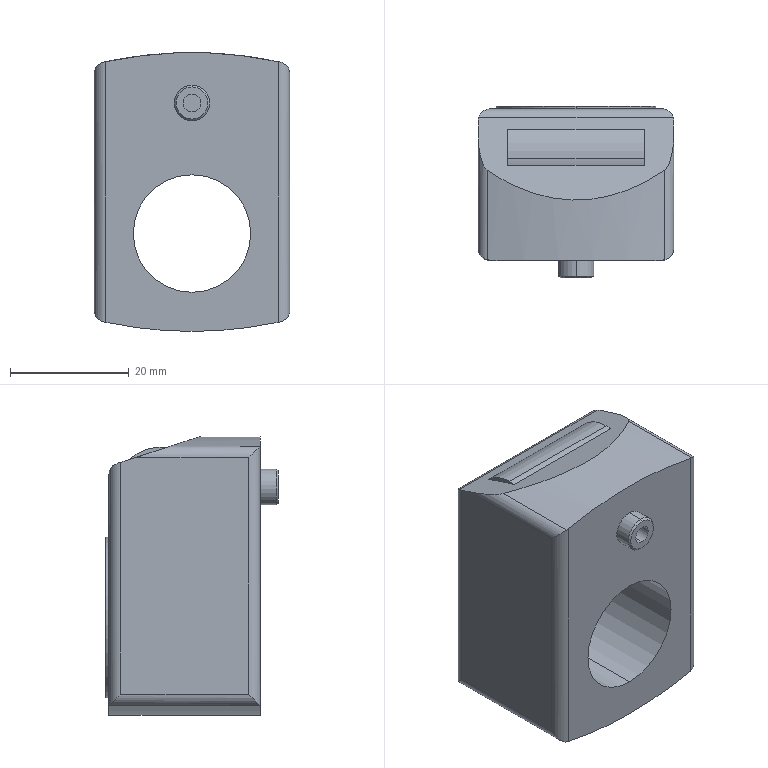Part | SolidWorks | features ICE 6, RefAxis 6, RevCut 3, 3DProfileFeature 2, Revolution 2, Extrusion 1 | 1 solid | 39 faces | box 33 x 29 x 47 mm | volume 29608 mm3 | cylinder 22 | plane 15 | cone 2 | commonest cylinder face diameters 4 x9 138.125 x3 3 x2 6 x2 14 x2 19.8 x2
STEP:
#1=CARTESIAN_POINT('',(11.5,3.069,28.669));
#2=VERTEX_POINT('',#1);
#3=CARTESIAN_POINT('',(11.5,2.,28.587));
#4=VERTEX_POINT('',#3);
#5=CARTESIAN_POINT('',(11.5,3.069,21.669));
#6=DIRECTION('',(1.,0.,0.));
#7=DIRECTION('',(0.,0.,-1.));
#8=AXIS2_PLACEMENT_3D('',#5,#6,#7);
#9=CIRCLE('',#8,7.);
#10=EDGE_CURVE('',#2,#4,#9,.T.);
#11=ORIENTED_EDGE('',*,*,#10,.F.);
#12=CARTESIAN_POINT('',(-11.5,3.069,28.669));
#13=VERTEX_POINT('',#12);
#14=CARTESIAN_POINT('',(11.5,3.069,28.669));
#15=DIRECTION('',(-1.,0.,0.));
#16=VECTOR('',#15,1000.);
#17=LINE('',#14,#16);
#18=EDGE_CURVE('',#2,#13,#17,.T.);
#19=ORIENTED_EDGE('',*,*,#18,.T.);
#20=CARTESIAN_POINT('',(-11.5,2.,28.587));
#21=VERTEX_POINT('',#20);
#22=CARTESIAN_POINT('',(-11.5,3.069,21.669));
#23=DIRECTION('',(1.,0.,0.));
#24=DIRECTION('',(0.,0.,-1.));
#25=AXIS2_PLACEMENT_3D('',#22,#23,#24);
#26=CIRCLE('',#25,7.);
#27=EDGE_CURVE('',#13,#21,#26,.T.);
#28=ORIENTED_EDGE('',*,*,#27,.T.);
#29=CARTESIAN_POINT('',(11.5,2.,28.587));
#30=DIRECTION('',(-1.,0.,0.));
#31=VECTOR('',#30,1000.);
#32=LINE('',#29,#31);
#33=EDGE_CURVE('',#4,#21,#32,.T.);
#34=ORIENTED_EDGE('',*,*,#33,.F.);
#35=EDGE_LOOP('',(#11,#19,#28,#34));
#36=FACE_OUTER_BOUND('',#35,.T.);
#37=CARTESIAN_POINT('',(11.5,3.069,21.669));
#38=DIRECTION('',(-1.,0.,0.));
#39=DIRECTION('',(0.,0.,1.));
#40=AXIS2_PLACEMENT_3D('',#37,#38,#39);
#41=CYLINDRICAL_SURFACE('',#40,7.);
#42=ADVANCED_FACE('',(#36),#41,.T.);
#43=CARTESIAN_POINT('',(0.,-17.,20.5));
#44=VERTEX_POINT('',#43);
#45=CARTESIAN_POINT('',(0.,-17.,23.5));
#46=VERTEX_POINT('',#45);
#47=CARTESIAN_POINT('',(0.,-17.,22.));
#48=DIRECTION('',(0.,1.,0.));
#49=DIRECTION('',(0.,0.,1.));
#50=AXIS2_PLACEMENT_3D('',#47,#48,#49);
#51=CIRCLE('',#50,1.5);
#52=EDGE_CURVE('',#44,#46,#51,.T.);
#53=ORIENTED_EDGE('',*,*,#52,.F.);
#54=CARTESIAN_POINT('',(0.,-12.,20.5));
#55=VERTEX_POINT('',#54);
#56=CARTESIAN_POINT('',(0.,-17.,20.5));
#57=DIRECTION('',(0.,1.,0.));
#58=VECTOR('',#57,1000.);
#59=LINE('',#56,#58);
#60=EDGE_CURVE('',#44,#55,#59,.T.);
#61=ORIENTED_EDGE('',*,*,#60,.T.);
#62=CARTESIAN_POINT('',(0.,-12.,23.5));
#63=VERTEX_POINT('',#62);
#64=CARTESIAN_POINT('',(0.,-12.,22.));
#65=DIRECTION('',(0.,1.,0.));
#66=DIRECTION('',(0.,0.,1.));
#67=AXIS2_PLACEMENT_3D('',#64,#65,#66);
#68=CIRCLE('',#67,1.5);
#69=EDGE_CURVE('',#55,#63,#68,.T.);
#70=ORIENTED_EDGE('',*,*,#69,.T.);
#71=CARTESIAN_POINT('',(0.,-17.,23.5));
#72=DIRECTION('',(0.,1.,0.));
#73=VECTOR('',#72,1000.);
#74=LINE('',#71,#73);
#75=EDGE_CURVE('',#46,#63,#74,.T.);
#76=ORIENTED_EDGE('',*,*,#75,.F.);
#77=EDGE_LOOP('',(#53,#61,#70,#76));
#78=FACE_OUTER_BOUND('',#77,.T.);
#79=CARTESIAN_POINT('',(0.,-17.,22.));
#80=DIRECTION('',(0.,1.,0.));
#81=DIRECTION('',(0.,0.,1.));
#82=AXIS2_PLACEMENT_3D('',#79,#80,#81);
#83=CYLINDRICAL_SURFACE('',#82,1.5);
#84=ADVANCED_FACE('',(#78),#83,.F.);
#85=CARTESIAN_POINT('',(0.,-17.,24.7));
#86=VERTEX_POINT('',#85);
#87=CARTESIAN_POINT('',(0.,-17.,19.3));
#88=VERTEX_POINT('',#87);
#89=CARTESIAN_POINT('',(0.,-17.,22.));
#90=DIRECTION('',(0.,1.,0.));
#91=DIRECTION('',(0.,0.,1.));
#92=AXIS2_PLACEMENT_3D('',#89,#90,#91);
#93=CIRCLE('',#92,2.7);
#94=EDGE_CURVE('',#86,#88,#93,.T.);
#95=ORIENTED_EDGE('',*,*,#94,.T.);
#96=CARTESIAN_POINT('',(0.,-16.7,19.));
#97=VERTEX_POINT('',#96);
#98=CARTESIAN_POINT('',(0.,-16.7,19.));
#99=DIRECTION('',(0.,0.7071,-0.7071));
#100=VECTOR('',#99,1000.);
#101=LINE('',#98,#100);
#102=EDGE_CURVE('',#88,#97,#101,.T.);
#103=ORIENTED_EDGE('',*,*,#102,.T.);
#104=CARTESIAN_POINT('',(0.,-16.7,25.));
#105=VERTEX_POINT('',#104);
#106=CARTESIAN_POINT('',(0.,-16.7,22.));
#107=DIRECTION('',(0.,1.,0.));
#108=DIRECTION('',(0.,0.,1.));
#109=AXIS2_PLACEMENT_3D('',#106,#107,#108);
#110=CIRCLE('',#109,3.);
#111=EDGE_CURVE('',#105,#97,#110,.T.);
#112=ORIENTED_EDGE('',*,*,#111,.F.);
#113=CARTESIAN_POINT('',(0.,-16.7,25.));
#114=DIRECTION('',(0.,0.7071,0.7071));
#115=VECTOR('',#114,1000.);
#116=LINE('',#113,#115);
#117=EDGE_CURVE('',#86,#105,#116,.T.);
#118=ORIENTED_EDGE('',*,*,#117,.F.);
#119=EDGE_LOOP('',(#95,#103,#112,#118));
#120=FACE_OUTER_BOUND('',#119,.T.);
#121=CARTESIAN_POINT('',(0.,-16.7,22.));
#122=DIRECTION('',(0.,1.,0.));
#123=DIRECTION('',(0.,0.,1.));
#124=AXIS2_PLACEMENT_3D('',#121,#122,#123);
#125=CONICAL_SURFACE('',#124,3.,0.7854);
#126=ADVANCED_FACE('',(#120),#125,.T.);
#127=ORIENTED_EDGE('',*,*,#111,.T.);
#128=CARTESIAN_POINT('',(0.,-14.,19.));
#129=VERTEX_POINT('',#128);
#130=CARTESIAN_POINT('',(0.,-10.,19.));
#131=DIRECTION('',(0.,1.,0.));
#132=VECTOR('',#131,1000.);
#133=LINE('',#130,#132);
#134=EDGE_CURVE('',#97,#129,#133,.T.);
#135=ORIENTED_EDGE('',*,*,#134,.T.);
#136=CARTESIAN_POINT('',(0.,-14.,25.));
#137=VERTEX_POINT('',#136);
#138=CARTESIAN_POINT('',(0.,-14.,22.));
#139=DIRECTION('',(0.,1.,0.));
#140=DIRECTION('',(0.,0.,1.));
#141=AXIS2_PLACEMENT_3D('',#138,#139,#140);
#142=CIRCLE('',#141,3.);
#143=EDGE_CURVE('',#137,#129,#142,.T.);
#144=ORIENTED_EDGE('',*,*,#143,.F.);
#145=CARTESIAN_POINT('',(0.,-10.,25.));
#146=DIRECTION('',(0.,1.,0.));
#147=VECTOR('',#146,1000.);
#148=LINE('',#145,#147);
#149=EDGE_CURVE('',#105,#137,#148,.T.);
#150=ORIENTED_EDGE('',*,*,#149,.F.);
#151=EDGE_LOOP('',(#127,#135,#144,#150));
#152=FACE_OUTER_BOUND('',#151,.T.);
#153=CARTESIAN_POINT('',(0.,-10.,22.));
#154=DIRECTION('',(0.,1.,0.));
#155=DIRECTION('',(0.,0.,1.));
#156=AXIS2_PLACEMENT_3D('',#153,#154,#155);
#157=CYLINDRICAL_SURFACE('',#156,3.);
#158=ADVANCED_FACE('',(#152),#157,.T.);
#159=CARTESIAN_POINT('',(0.,11.5,13.5));
#160=VERTEX_POINT('',#159);
#161=CARTESIAN_POINT('',(0.,11.5,-13.5));
#162=VERTEX_POINT('',#161);
#163=CARTESIAN_POINT('',(0.,11.5,0.));
#164=DIRECTION('',(0.,1.,0.));
#165=DIRECTION('',(0.,0.,1.));
#166=AXIS2_PLACEMENT_3D('',#163,#164,#165);
#167=CIRCLE('',#166,13.5);
#168=EDGE_CURVE('',#160,#162,#167,.T.);
#169=ORIENTED_EDGE('',*,*,#168,.T.);
#170=CARTESIAN_POINT('',(0.,12.,-13.5));
#171=VERTEX_POINT('',#170);
#172=CARTESIAN_POINT('',(0.,5.,-13.5));
#173=DIRECTION('',(0.,1.,0.));
#174=VECTOR('',#173,1000.);
#175=LINE('',#172,#174);
#176=EDGE_CURVE('',#162,#171,#175,.T.);
#177=ORIENTED_EDGE('',*,*,#176,.T.);
#178=CARTESIAN_POINT('',(0.,12.,13.5));
#179=VERTEX_POINT('',#178);
#180=CARTESIAN_POINT('',(0.,12.,0.));
#181=DIRECTION('',(0.,1.,0.));
#182=DIRECTION('',(0.,0.,1.));
#183=AXIS2_PLACEMENT_3D('',#180,#181,#182);
#184=CIRCLE('',#183,13.5);
#185=EDGE_CURVE('',#179,#171,#184,.T.);
#186=ORIENTED_EDGE('',*,*,#185,.F.);
#187=CARTESIAN_POINT('',(0.,5.,13.5));
#188=DIRECTION('',(0.,1.,0.));
#189=VECTOR('',#188,1000.);
#190=LINE('',#187,#189);
#191=EDGE_CURVE('',#160,#179,#190,.T.);
#192=ORIENTED_EDGE('',*,*,#191,.F.);
#193=EDGE_LOOP('',(#169,#177,#186,#192));
#194=FACE_OUTER_BOUND('',#193,.T.);
#195=CARTESIAN_POINT('',(0.,5.,0.));
#196=DIRECTION('',(0.,1.,0.));
#197=DIRECTION('',(0.,0.,1.));
#198=AXIS2_PLACEMENT_3D('',#195,#196,#197);
#199=CYLINDRICAL_SURFACE('',#198,13.5);
#200=ADVANCED_FACE('',(#194),#199,.T.);
#201=CARTESIAN_POINT('',(0.,-14.,9.9));
#202=VERTEX_POINT('',#201);
#203=CARTESIAN_POINT('',(0.,-14.,-9.9));
#204=VERTEX_POINT('',#203);
#205=CARTESIAN_POINT('',(0.,-14.,0.));
#206=DIRECTION('',(0.,-1.,0.));
#207=DIRECTION('',(0.,0.,-1.));
#208=AXIS2_PLACEMENT_3D('',#205,#206,#207);
#209=CIRCLE('',#208,9.9);
#210=EDGE_CURVE('',#202,#204,#209,.T.);
#211=ORIENTED_EDGE('',*,*,#210,.T.);
#212=CARTESIAN_POINT('',(0.,12.,-9.9));
#213=VERTEX_POINT('',#212);
#214=CARTESIAN_POINT('',(0.,12.,-9.9));
#215=DIRECTION('',(0.,1.,0.));
#216=VECTOR('',#215,1000.);
#217=LINE('',#214,#216);
#218=EDGE_CURVE('',#204,#213,#217,.T.);
#219=ORIENTED_EDGE('',*,*,#218,.T.);
#220=CARTESIAN_POINT('',(0.,12.,9.9));
#221=VERTEX_POINT('',#220);
#222=CARTESIAN_POINT('',(0.,12.,0.));
#223=DIRECTION('',(0.,1.,0.));
#224=DIRECTION('',(0.,0.,1.));
#225=AXIS2_PLACEMENT_3D('',#222,#223,#224);
#226=CIRCLE('',#225,9.9);
#227=EDGE_CURVE('',#213,#221,#226,.T.);
#228=ORIENTED_EDGE('',*,*,#227,.T.);
#229=CARTESIAN_POINT('',(0.,12.,9.9));
#230=DIRECTION('',(0.,1.,0.));
#231=VECTOR('',#230,1000.);
#232=LINE('',#229,#231);
#233=EDGE_CURVE('',#202,#221,#232,.T.);
#234=ORIENTED_EDGE('',*,*,#233,.F.);
#235=EDGE_LOOP('',(#211,#219,#228,#234));
#236=FACE_OUTER_BOUND('',#235,.T.);
#237=CARTESIAN_POINT('',(0.,12.,0.));
#238=DIRECTION('',(0.,1.,0.));
#239=DIRECTION('',(0.,0.,1.));
#240=AXIS2_PLACEMENT_3D('',#237,#238,#239);
#241=CYLINDRICAL_SURFACE('',#240,9.9);
#242=ADVANCED_FACE('',(#236),#241,.F.);
#243=CARTESIAN_POINT('',(0.,11.5,-16.5));
#244=VERTEX_POINT('',#243);
#245=CARTESIAN_POINT('',(-14.5,11.5,-14.961));
#246=VERTEX_POINT('',#245);
#247=CARTESIAN_POINT('',(0.,11.5,52.563));
#248=DIRECTION('',(0.,1.,0.));
#249=DIRECTION('',(0.,0.,1.));
#250=AXIS2_PLACEMENT_3D('',#247,#248,#249);
#251=CIRCLE('',#250,69.063);
#252=EDGE_CURVE('',#244,#246,#251,.T.);
#253=ORIENTED_EDGE('',*,*,#252,.F.);
#254=CARTESIAN_POINT('',(0.,-14.,-16.5));
#255=VERTEX_POINT('',#254);
#256=CARTESIAN_POINT('',(0.,11.5,-16.5));
#257=DIRECTION('',(0.,-1.,0.));
#258=VECTOR('',#257,1000.);
#259=LINE('',#256,#258);
#260=EDGE_CURVE('',#244,#255,#259,.T.);
#261=ORIENTED_EDGE('',*,*,#260,.T.);
#262=CARTESIAN_POINT('',(-14.5,-14.,-14.961));
#263=VERTEX_POINT('',#262);
#264=CARTESIAN_POINT('',(0.,-14.,52.563));
#265=DIRECTION('',(0.,1.,0.));
#266=DIRECTION('',(0.,0.,1.));
#267=AXIS2_PLACEMENT_3D('',#264,#265,#266);
#268=CIRCLE('',#267,69.063);
#269=EDGE_CURVE('',#255,#263,#268,.T.);
#270=ORIENTED_EDGE('',*,*,#269,.T.);
#271=CARTESIAN_POINT('',(-14.932,-13.953,-14.866));
#272=VERTEX_POINT('',#271);
#273=CARTESIAN_POINT('',(-14.932,-13.953,-14.866));
#274=CARTESIAN_POINT('',(-14.79,-13.984,-14.898));
#275=CARTESIAN_POINT('',(-14.646,-14.,-14.929));
#276=CARTESIAN_POINT('',(-14.5,-14.,-14.961));
#277=B_SPLINE_CURVE_WITH_KNOTS('',3,(#273,#274,#275,#276),.UNSPECIFIED.,.F.,.F.,(4,4),(0.,0.0004451),.UNSPECIFIED.);
#278=EDGE_CURVE('',#272,#263,#277,.T.);
#279=ORIENTED_EDGE('',*,*,#278,.F.);
#280=CARTESIAN_POINT('',(-14.932,11.453,-14.866));
#281=VERTEX_POINT('',#280);
#282=CARTESIAN_POINT('',(-14.932,11.5,-14.866));
#283=DIRECTION('',(0.,-1.,0.));
#284=VECTOR('',#283,1000.);
#285=LINE('',#282,#284);
#286=EDGE_CURVE('',#281,#272,#285,.T.);
#287=ORIENTED_EDGE('',*,*,#286,.F.);
#288=CARTESIAN_POINT('',(-14.5,11.5,-14.961));
#289=CARTESIAN_POINT('',(-14.646,11.5,-14.929));
#290=CARTESIAN_POINT('',(-14.79,11.484,-14.898));
#291=CARTESIAN_POINT('',(-14.932,11.453,-14.866));
#292=B_SPLINE_CURVE_WITH_KNOTS('',3,(#288,#289,#290,#291),.UNSPECIFIED.,.F.,.F.,(4,4),(0.,0.0004451),.UNSPECIFIED.);
#293=EDGE_CURVE('',#246,#281,#292,.T.);
#294=ORIENTED_EDGE('',*,*,#293,.F.);
#295=EDGE_LOOP('',(#253,#261,#270,#279,#287,#294));
#296=FACE_OUTER_BOUND('',#295,.T.);
#297=CARTESIAN_POINT('',(0.,11.5,52.563));
#298=DIRECTION('',(0.,-1.,0.));
#299=DIRECTION('',(0.,0.,-1.));
#300=AXIS2_PLACEMENT_3D('',#297,#298,#299);
#301=CYLINDRICAL_SURFACE('',#300,69.063);
#302=ADVANCED_FACE('',(#296),#301,.T.);
#303=ORIENTED_EDGE('',*,*,#94,.F.);
#304=CARTESIAN_POINT('',(0.,-17.,22.));
#305=DIRECTION('',(0.,1.,0.));
#306=DIRECTION('',(0.,0.,1.));
#307=AXIS2_PLACEMENT_3D('',#304,#305,#306);
#308=CIRCLE('',#307,2.7);
#309=EDGE_CURVE('',#88,#86,#308,.T.);
#310=ORIENTED_EDGE('',*,*,#309,.F.);
#311=EDGE_LOOP('',(#303,#310));
#312=FACE_OUTER_BOUND('',#311,.T.);
#313=CARTESIAN_POINT('',(0.,-17.,22.));
#314=DIRECTION('',(0.,1.,0.));
#315=DIRECTION('',(0.,0.,1.));
#316=AXIS2_PLACEMENT_3D('',#313,#314,#315);
#317=CIRCLE('',#316,1.5);
#318=EDGE_CURVE('',#46,#44,#317,.T.);
#319=ORIENTED_EDGE('',*,*,#318,.T.);
#320=ORIENTED_EDGE('',*,*,#52,.T.);
#321=EDGE_LOOP('',(#319,#320));
#322=FACE_BOUND('',#321,.T.);
#323=CARTESIAN_POINT('',(0.,-17.,22.));
#324=DIRECTION('',(0.,-1.,0.));
#325=DIRECTION('',(0.,0.,-1.));
#326=AXIS2_PLACEMENT_3D('',#323,#324,#325);
#327=PLANE('',#326);
#328=ADVANCED_FACE('',(#312,#322),#327,.T.);
#329=ORIENTED_EDGE('',*,*,#143,.T.);
#330=CARTESIAN_POINT('',(0.,-14.,22.));
#331=DIRECTION('',(0.,1.,0.));
#332=DIRECTION('',(0.,0.,1.));
#333=AXIS2_PLACEMENT_3D('',#330,#331,#332);
#334=CIRCLE('',#333,3.);
#335=EDGE_CURVE('',#129,#137,#334,.T.);
#336=ORIENTED_EDGE('',*,*,#335,.T.);
#337=EDGE_LOOP('',(#329,#336));
#338=FACE_BOUND('',#337,.T.);
#339=CARTESIAN_POINT('',(14.5,-14.,-14.961));
#340=VERTEX_POINT('',#339);
#341=CARTESIAN_POINT('',(14.5,-14.,28.961));
#342=VERTEX_POINT('',#341);
#343=CARTESIAN_POINT('',(14.5,-14.,-35.));
#344=DIRECTION('',(0.,0.,1.));
#345=VECTOR('',#344,1000.);
#346=LINE('',#343,#345);
#347=EDGE_CURVE('',#340,#342,#346,.T.);
#348=ORIENTED_EDGE('',*,*,#347,.T.);
#349=CARTESIAN_POINT('',(-14.5,-14.,28.961));
#350=VERTEX_POINT('',#349);
#351=CARTESIAN_POINT('',(0.,-14.,-38.563));
#352=DIRECTION('',(0.,1.,0.));
#353=DIRECTION('',(0.,0.,1.));
#354=AXIS2_PLACEMENT_3D('',#351,#352,#353);
#355=CIRCLE('',#354,69.063);
#356=EDGE_CURVE('',#350,#342,#355,.T.);
#357=ORIENTED_EDGE('',*,*,#356,.F.);
#358=CARTESIAN_POINT('',(-14.5,-14.,-35.));
#359=DIRECTION('',(0.,0.,1.));
#360=VECTOR('',#359,1000.);
#361=LINE('',#358,#360);
#362=EDGE_CURVE('',#263,#350,#361,.T.);
#363=ORIENTED_EDGE('',*,*,#362,.F.);
#364=ORIENTED_EDGE('',*,*,#269,.F.);
#365=CARTESIAN_POINT('',(0.,-14.,52.563));
#366=DIRECTION('',(0.,1.,0.));
#367=DIRECTION('',(0.,0.,1.));
#368=AXIS2_PLACEMENT_3D('',#365,#366,#367);
#369=CIRCLE('',#368,69.063);
#370=EDGE_CURVE('',#340,#255,#369,.T.);
#371=ORIENTED_EDGE('',*,*,#370,.F.);
#372=EDGE_LOOP('',(#348,#357,#363,#364,#371));
#373=FACE_OUTER_BOUND('',#372,.T.);
#374=ORIENTED_EDGE('',*,*,#210,.F.);
#375=CARTESIAN_POINT('',(0.,-14.,0.));
#376=DIRECTION('',(0.,-1.,0.));
#377=DIRECTION('',(0.,0.,-1.));
#378=AXIS2_PLACEMENT_3D('',#375,#376,#377);
#379=CIRCLE('',#378,9.9);
#380=EDGE_CURVE('',#204,#202,#379,.T.);
#381=ORIENTED_EDGE('',*,*,#380,.F.);
#382=EDGE_LOOP('',(#374,#381));
#383=FACE_BOUND('',#382,.T.);
#384=CARTESIAN_POINT('',(-14.5,-14.,-12.914));
#385=DIRECTION('',(0.,1.,0.));
#386=DIRECTION('',(0.,0.,1.));
#387=AXIS2_PLACEMENT_3D('',#384,#385,#386);
#388=PLANE('',#387);
#389=ADVANCED_FACE('',(#338,#373,#383),#388,.F.);
#390=CARTESIAN_POINT('',(-16.5,9.5,-12.914));
#391=VERTEX_POINT('',#390);
#392=CARTESIAN_POINT('',(-14.932,11.453,-14.866));
#393=CARTESIAN_POINT('',(-15.888,11.241,-14.655));
#394=CARTESIAN_POINT('',(-16.5,10.478,-13.892));
#395=CARTESIAN_POINT('',(-16.5,9.5,-12.914));
#396=(BOUNDED_CURVE()B_SPLINE_CURVE(3,(#392,#393,#394,#395),.UNSPECIFIED.,.F.,.F.)B_SPLINE_CURVE_WITH_KNOTS((4,4),(3.36,4.712),.UNSPECIFIED.)CURVE()GEOMETRIC_REPRESENTATION_ITEM()RATIONAL_B_SPLINE_CURVE((1.,0.8532,0.8532,1.))REPRESENTATION_ITEM(''));
#397=EDGE_CURVE('',#281,#391,#396,.T.);
#398=ORIENTED_EDGE('',*,*,#397,.F.);
#399=ORIENTED_EDGE('',*,*,#286,.T.);
#400=CARTESIAN_POINT('',(-16.5,-12.,-12.914));
#401=VERTEX_POINT('',#400);
#402=CARTESIAN_POINT('',(-16.5,-12.,-12.914));
#403=CARTESIAN_POINT('',(-16.5,-12.978,-13.892));
#404=CARTESIAN_POINT('',(-15.888,-13.741,-14.655));
#405=CARTESIAN_POINT('',(-14.932,-13.953,-14.866));
#406=(BOUNDED_CURVE()B_SPLINE_CURVE(3,(#402,#403,#404,#405),.UNSPECIFIED.,.F.,.F.)B_SPLINE_CURVE_WITH_KNOTS((4,4),(4.712,6.065),.UNSPECIFIED.)CURVE()GEOMETRIC_REPRESENTATION_ITEM()RATIONAL_B_SPLINE_CURVE((1.,0.8532,0.8532,1.))REPRESENTATION_ITEM(''));
#407=EDGE_CURVE('',#401,#272,#406,.T.);
#408=ORIENTED_EDGE('',*,*,#407,.F.);
#409=CARTESIAN_POINT('',(-16.5,11.5,-12.914));
#410=DIRECTION('',(0.,-1.,0.));
#411=VECTOR('',#410,1000.);
#412=LINE('',#409,#411);
#413=EDGE_CURVE('',#391,#401,#412,.T.);
#414=ORIENTED_EDGE('',*,*,#413,.F.);
#415=EDGE_LOOP('',(#398,#399,#408,#414));
#416=FACE_OUTER_BOUND('',#415,.T.);
#417=CARTESIAN_POINT('',(-14.5,11.5,-12.914));
#418=DIRECTION('',(0.,-1.,0.));
#419=DIRECTION('',(0.,0.,-1.));
#420=AXIS2_PLACEMENT_3D('',#417,#418,#419);
#421=CYLINDRICAL_SURFACE('',#420,2.);
#422=ADVANCED_FACE('',(#416),#421,.T.);
#423=CARTESIAN_POINT('',(-16.5,7.149,26.914));
#424=VERTEX_POINT('',#423);
#425=CARTESIAN_POINT('',(-16.5,-12.,26.914));
#426=VERTEX_POINT('',#425);
#427=CARTESIAN_POINT('',(-16.5,11.5,26.914));
#428=DIRECTION('',(0.,-1.,0.));
#429=VECTOR('',#428,1000.);
#430=LINE('',#427,#429);
#431=EDGE_CURVE('',#424,#426,#430,.T.);
#432=ORIENTED_EDGE('',*,*,#431,.F.);
#433=CARTESIAN_POINT('',(-16.5,9.5,26.15));
#434=VERTEX_POINT('',#433);
#435=CARTESIAN_POINT('',(-16.5,22.789,21.832));
#436=DIRECTION('',(0.,0.9511,-0.309));
#437=VECTOR('',#436,1000.);
#438=LINE('',#435,#437);
#439=EDGE_CURVE('',#424,#434,#438,.T.);
#440=ORIENTED_EDGE('',*,*,#439,.T.);
#441=CARTESIAN_POINT('',(-16.5,9.5,-35.));
#442=DIRECTION('',(0.,0.,1.));
#443=VECTOR('',#442,1000.);
#444=LINE('',#441,#443);
#445=EDGE_CURVE('',#391,#434,#444,.T.);
#446=ORIENTED_EDGE('',*,*,#445,.F.);
#447=ORIENTED_EDGE('',*,*,#413,.T.);
#448=CARTESIAN_POINT('',(-16.5,-12.,-35.));
#449=DIRECTION('',(0.,0.,1.));
#450=VECTOR('',#449,1000.);
#451=LINE('',#448,#450);
#452=EDGE_CURVE('',#401,#426,#451,.T.);
#453=ORIENTED_EDGE('',*,*,#452,.T.);
#454=EDGE_LOOP('',(#432,#440,#446,#447,#453));
#455=FACE_OUTER_BOUND('',#454,.T.);
#456=CARTESIAN_POINT('',(-16.5,11.5,-12.914));
#457=DIRECTION('',(1.,0.,0.));
#458=DIRECTION('',(0.,0.,-1.));
#459=AXIS2_PLACEMENT_3D('',#456,#457,#458);
#460=PLANE('',#459);
#461=ADVANCED_FACE('',(#455),#460,.F.);
#462=CARTESIAN_POINT('',(-14.932,1.139,28.866));
#463=VERTEX_POINT('',#462);
#464=CARTESIAN_POINT('',(-14.932,-13.953,28.866));
#465=VERTEX_POINT('',#464);
#466=CARTESIAN_POINT('',(-14.932,11.5,28.866));
#467=DIRECTION('',(0.,-1.,0.));
#468=VECTOR('',#467,1000.);
#469=LINE('',#466,#468);
#470=EDGE_CURVE('',#463,#465,#469,.T.);
#471=ORIENTED_EDGE('',*,*,#470,.F.);
#472=CARTESIAN_POINT('',(-14.932,1.139,28.866));
#473=CARTESIAN_POINT('',(-15.888,1.79,28.655));
#474=CARTESIAN_POINT('',(-16.5,4.138,27.892));
#475=CARTESIAN_POINT('',(-16.5,7.149,26.914));
#476=(BOUNDED_CURVE()B_SPLINE_CURVE(3,(#472,#473,#474,#475),.UNSPECIFIED.,.F.,.F.)B_SPLINE_CURVE_WITH_KNOTS((4,4),(0.2179,1.571),.UNSPECIFIED.)CURVE()GEOMETRIC_REPRESENTATION_ITEM()RATIONAL_B_SPLINE_CURVE((1.,0.8532,0.8532,1.))REPRESENTATION_ITEM(''));
#477=EDGE_CURVE('',#463,#424,#476,.T.);
#478=ORIENTED_EDGE('',*,*,#477,.T.);
#479=ORIENTED_EDGE('',*,*,#431,.T.);
#480=CARTESIAN_POINT('',(-14.932,-13.953,28.866));
#481=CARTESIAN_POINT('',(-15.888,-13.741,28.655));
#482=CARTESIAN_POINT('',(-16.5,-12.978,27.892));
#483=CARTESIAN_POINT('',(-16.5,-12.,26.914));
#484=(BOUNDED_CURVE()B_SPLINE_CURVE(3,(#480,#481,#482,#483),.UNSPECIFIED.,.F.,.F.)B_SPLINE_CURVE_WITH_KNOTS((4,4),(0.2179,1.571),.UNSPECIFIED.)CURVE()GEOMETRIC_REPRESENTATION_ITEM()RATIONAL_B_SPLINE_CURVE((1.,0.8532,0.8532,1.))REPRESENTATION_ITEM(''));
#485=EDGE_CURVE('',#465,#426,#484,.T.);
#486=ORIENTED_EDGE('',*,*,#485,.F.);
#487=EDGE_LOOP('',(#471,#478,#479,#486));
#488=FACE_OUTER_BOUND('',#487,.T.);
#489=CARTESIAN_POINT('',(-14.5,11.5,26.914));
#490=DIRECTION('',(0.,-1.,0.));
#491=DIRECTION('',(0.,0.,-1.));
#492=AXIS2_PLACEMENT_3D('',#489,#490,#491);
#493=CYLINDRICAL_SURFACE('',#492,2.);
#494=ADVANCED_FACE('',(#488),#493,.T.);
#495=CARTESIAN_POINT('',(14.932,1.139,28.866));
#496=VERTEX_POINT('',#495);
#497=CARTESIAN_POINT('',(14.932,-13.953,28.866));
#498=VERTEX_POINT('',#497);
#499=CARTESIAN_POINT('',(14.932,11.5,28.866));
#500=DIRECTION('',(0.,-1.,0.));
#501=VECTOR('',#500,1000.);
#502=LINE('',#499,#501);
#503=EDGE_CURVE('',#496,#498,#502,.T.);
#504=ORIENTED_EDGE('',*,*,#503,.F.);
#505=CARTESIAN_POINT('',(14.932,1.139,28.866));
#506=CARTESIAN_POINT('',(5.057,-5.591,31.053));
#507=CARTESIAN_POINT('',(-5.057,-5.591,31.053));
#508=CARTESIAN_POINT('',(-14.932,1.139,28.866));
#509=(BOUNDED_CURVE()B_SPLINE_CURVE(3,(#505,#506,#507,#508),.UNSPECIFIED.,.F.,.F.)B_SPLINE_CURVE_WITH_KNOTS((4,4),(6.065,6.501),.UNSPECIFIED.)CURVE()GEOMETRIC_REPRESENTATION_ITEM()RATIONAL_B_SPLINE_CURVE((1.,0.9842,0.9842,1.))REPRESENTATION_ITEM(''));
#510=EDGE_CURVE('',#496,#463,#509,.T.);
#511=ORIENTED_EDGE('',*,*,#510,.T.);
#512=ORIENTED_EDGE('',*,*,#470,.T.);
#513=CARTESIAN_POINT('',(-14.5,-14.,28.961));
#514=CARTESIAN_POINT('',(-14.646,-14.,28.929));
#515=CARTESIAN_POINT('',(-14.79,-13.984,28.898));
#516=CARTESIAN_POINT('',(-14.932,-13.953,28.866));
#517=B_SPLINE_CURVE_WITH_KNOTS('',3,(#513,#514,#515,#516),.UNSPECIFIED.,.F.,.F.,(4,4),(0.,0.0004451),.UNSPECIFIED.);
#518=EDGE_CURVE('',#350,#465,#517,.T.);
#519=ORIENTED_EDGE('',*,*,#518,.F.);
#520=ORIENTED_EDGE('',*,*,#356,.T.);
#521=CARTESIAN_POINT('',(14.932,-13.953,28.866));
#522=CARTESIAN_POINT('',(14.79,-13.984,28.898));
#523=CARTESIAN_POINT('',(14.646,-14.,28.929));
#524=CARTESIAN_POINT('',(14.5,-14.,28.961));
#525=B_SPLINE_CURVE_WITH_KNOTS('',3,(#521,#522,#523,#524),.UNSPECIFIED.,.F.,.F.,(4,4),(0.,0.0004451),.UNSPECIFIED.);
#526=EDGE_CURVE('',#498,#342,#525,.T.);
#527=ORIENTED_EDGE('',*,*,#526,.F.);
#528=EDGE_LOOP('',(#504,#511,#512,#519,#520,#527));
#529=FACE_OUTER_BOUND('',#528,.T.);
#530=CARTESIAN_POINT('',(0.,11.5,-38.563));
#531=DIRECTION('',(0.,-1.,0.));
#532=DIRECTION('',(0.,0.,-1.));
#533=AXIS2_PLACEMENT_3D('',#530,#531,#532);
#534=CYLINDRICAL_SURFACE('',#533,69.063);
#535=ADVANCED_FACE('',(#529),#534,.T.);
#536=CARTESIAN_POINT('',(16.5,7.149,26.914));
#537=VERTEX_POINT('',#536);
#538=CARTESIAN_POINT('',(16.5,-12.,26.914));
#539=VERTEX_POINT('',#538);
#540=CARTESIAN_POINT('',(16.5,11.5,26.914));
#541=DIRECTION('',(0.,-1.,0.));
#542=VECTOR('',#541,1000.);
#543=LINE('',#540,#542);
#544=EDGE_CURVE('',#537,#539,#543,.T.);
#545=ORIENTED_EDGE('',*,*,#544,.F.);
#546=CARTESIAN_POINT('',(16.5,7.149,26.914));
#547=CARTESIAN_POINT('',(16.5,4.138,27.892));
#548=CARTESIAN_POINT('',(15.888,1.79,28.655));
#549=CARTESIAN_POINT('',(14.932,1.139,28.866));
#550=(BOUNDED_CURVE()B_SPLINE_CURVE(3,(#546,#547,#548,#549),.UNSPECIFIED.,.F.,.T.)B_SPLINE_CURVE_WITH_KNOTS((4,4),(4.712,6.065),.UNSPECIFIED.)CURVE()GEOMETRIC_REPRESENTATION_ITEM()RATIONAL_B_SPLINE_CURVE((1.,0.8532,0.8532,1.))REPRESENTATION_ITEM(''));
#551=EDGE_CURVE('',#537,#496,#550,.T.);
#552=ORIENTED_EDGE('',*,*,#551,.T.);
#553=ORIENTED_EDGE('',*,*,#503,.T.);
#554=CARTESIAN_POINT('',(16.5,-12.,26.914));
#555=CARTESIAN_POINT('',(16.5,-12.978,27.892));
#556=CARTESIAN_POINT('',(15.888,-13.741,28.655));
#557=CARTESIAN_POINT('',(14.932,-13.953,28.866));
#558=(BOUNDED_CURVE()B_SPLINE_CURVE(3,(#554,#555,#556,#557),.UNSPECIFIED.,.F.,.F.)B_SPLINE_CURVE_WITH_KNOTS((4,4),(4.712,6.065),.UNSPECIFIED.)CURVE()GEOMETRIC_REPRESENTATION_ITEM()RATIONAL_B_SPLINE_CURVE((1.,0.8532,0.8532,1.))REPRESENTATION_ITEM(''));
#559=EDGE_CURVE('',#539,#498,#558,.T.);
#560=ORIENTED_EDGE('',*,*,#559,.F.);
#561=EDGE_LOOP('',(#545,#552,#553,#560));
#562=FACE_OUTER_BOUND('',#561,.T.);
#563=CARTESIAN_POINT('',(14.5,11.5,26.914));
#564=DIRECTION('',(0.,-1.,0.));
#565=DIRECTION('',(0.,0.,-1.));
#566=AXIS2_PLACEMENT_3D('',#563,#564,#565);
#567=CYLINDRICAL_SURFACE('',#566,2.);
#568=ADVANCED_FACE('',(#562),#567,.T.);
#569=CARTESIAN_POINT('',(16.5,9.5,-12.914));
#570=VERTEX_POINT('',#569);
#571=CARTESIAN_POINT('',(16.5,9.5,26.15));
#572=VERTEX_POINT('',#571);
#573=CARTESIAN_POINT('',(16.5,9.5,-35.));
#574=DIRECTION('',(0.,0.,1.));
#575=VECTOR('',#574,1000.);
#576=LINE('',#573,#575);
#577=EDGE_CURVE('',#570,#572,#576,.T.);
#578=ORIENTED_EDGE('',*,*,#577,.T.);
#579=CARTESIAN_POINT('',(16.5,11.085,25.635));
#580=DIRECTION('',(0.,-0.9511,0.309));
#581=VECTOR('',#580,1000.);
#582=LINE('',#579,#581);
#583=EDGE_CURVE('',#572,#537,#582,.T.);
#584=ORIENTED_EDGE('',*,*,#583,.T.);
#585=ORIENTED_EDGE('',*,*,#544,.T.);
#586=CARTESIAN_POINT('',(16.5,-12.,-12.914));
#587=VERTEX_POINT('',#586);
#588=CARTESIAN_POINT('',(16.5,-12.,-35.));
#589=DIRECTION('',(0.,0.,1.));
#590=VECTOR('',#589,1000.);
#591=LINE('',#588,#590);
#592=EDGE_CURVE('',#587,#539,#591,.T.);
#593=ORIENTED_EDGE('',*,*,#592,.F.);
#594=CARTESIAN_POINT('',(16.5,11.5,-12.914));
#595=DIRECTION('',(0.,-1.,0.));
#596=VECTOR('',#595,1000.);
#597=LINE('',#594,#596);
#598=EDGE_CURVE('',#570,#587,#597,.T.);
#599=ORIENTED_EDGE('',*,*,#598,.F.);
#600=EDGE_LOOP('',(#578,#584,#585,#593,#599));
#601=FACE_OUTER_BOUND('',#600,.T.);
#602=CARTESIAN_POINT('',(16.5,11.5,26.914));
#603=DIRECTION('',(-1.,0.,0.));
#604=DIRECTION('',(0.,0.,1.));
#605=AXIS2_PLACEMENT_3D('',#602,#603,#604);
#606=PLANE('',#605);
#607=ADVANCED_FACE('',(#601),#606,.F.);
#608=CARTESIAN_POINT('',(14.932,11.453,-14.866));
#609=VERTEX_POINT('',#608);
#610=CARTESIAN_POINT('',(16.5,9.5,-12.914));
#611=CARTESIAN_POINT('',(16.5,10.478,-13.892));
#612=CARTESIAN_POINT('',(15.888,11.241,-14.655));
#613=CARTESIAN_POINT('',(14.932,11.453,-14.866));
#614=(BOUNDED_CURVE()B_SPLINE_CURVE(3,(#610,#611,#612,#613),.UNSPECIFIED.,.F.,.F.)B_SPLINE_CURVE_WITH_KNOTS((4,4),(1.571,2.924),.UNSPECIFIED.)CURVE()GEOMETRIC_REPRESENTATION_ITEM()RATIONAL_B_SPLINE_CURVE((1.,0.8532,0.8532,1.))REPRESENTATION_ITEM(''));
#615=EDGE_CURVE('',#570,#609,#614,.T.);
#616=ORIENTED_EDGE('',*,*,#615,.F.);
#617=ORIENTED_EDGE('',*,*,#598,.T.);
#618=CARTESIAN_POINT('',(14.932,-13.953,-14.866));
#619=VERTEX_POINT('',#618);
#620=CARTESIAN_POINT('',(14.932,-13.953,-14.866));
#621=CARTESIAN_POINT('',(15.888,-13.741,-14.655));
#622=CARTESIAN_POINT('',(16.5,-12.978,-13.892));
#623=CARTESIAN_POINT('',(16.5,-12.,-12.914));
#624=(BOUNDED_CURVE()B_SPLINE_CURVE(3,(#620,#621,#622,#623),.UNSPECIFIED.,.F.,.F.)B_SPLINE_CURVE_WITH_KNOTS((4,4),(0.2179,1.571),.UNSPECIFIED.)CURVE()GEOMETRIC_REPRESENTATION_ITEM()RATIONAL_B_SPLINE_CURVE((1.,0.8532,0.8532,1.))REPRESENTATION_ITEM(''));
#625=EDGE_CURVE('',#619,#587,#624,.T.);
#626=ORIENTED_EDGE('',*,*,#625,.F.);
#627=CARTESIAN_POINT('',(14.932,11.5,-14.866));
#628=DIRECTION('',(0.,-1.,0.));
#629=VECTOR('',#628,1000.);
#630=LINE('',#627,#629);
#631=EDGE_CURVE('',#609,#619,#630,.T.);
#632=ORIENTED_EDGE('',*,*,#631,.F.);
#633=EDGE_LOOP('',(#616,#617,#626,#632));
#634=FACE_OUTER_BOUND('',#633,.T.);
#635=CARTESIAN_POINT('',(14.5,11.5,-12.914));
#636=DIRECTION('',(0.,-1.,0.));
#637=DIRECTION('',(0.,0.,-1.));
#638=AXIS2_PLACEMENT_3D('',#635,#636,#637);
#639=CYLINDRICAL_SURFACE('',#638,2.);
#640=ADVANCED_FACE('',(#634),#639,.T.);
#641=ORIENTED_EDGE('',*,*,#260,.F.);
#642=CARTESIAN_POINT('',(14.5,11.5,-14.961));
#643=VERTEX_POINT('',#642);
#644=CARTESIAN_POINT('',(0.,11.5,52.563));
#645=DIRECTION('',(0.,1.,0.));
#646=DIRECTION('',(0.,0.,1.));
#647=AXIS2_PLACEMENT_3D('',#644,#645,#646);
#648=CIRCLE('',#647,69.063);
#649=EDGE_CURVE('',#643,#244,#648,.T.);
#650=ORIENTED_EDGE('',*,*,#649,.F.);
#651=CARTESIAN_POINT('',(14.932,11.453,-14.866));
#652=CARTESIAN_POINT('',(14.79,11.484,-14.898));
#653=CARTESIAN_POINT('',(14.646,11.5,-14.929));
#654=CARTESIAN_POINT('',(14.5,11.5,-14.961));
#655=B_SPLINE_CURVE_WITH_KNOTS('',3,(#651,#652,#653,#654),.UNSPECIFIED.,.F.,.F.,(4,4),(0.,0.0004451),.UNSPECIFIED.);
#656=EDGE_CURVE('',#609,#643,#655,.T.);
#657=ORIENTED_EDGE('',*,*,#656,.F.);
#658=ORIENTED_EDGE('',*,*,#631,.T.);
#659=CARTESIAN_POINT('',(14.5,-14.,-14.961));
#660=CARTESIAN_POINT('',(14.646,-14.,-14.929));
#661=CARTESIAN_POINT('',(14.79,-13.984,-14.898));
#662=CARTESIAN_POINT('',(14.932,-13.953,-14.866));
#663=B_SPLINE_CURVE_WITH_KNOTS('',3,(#659,#660,#661,#662),.UNSPECIFIED.,.F.,.F.,(4,4),(0.,0.0004451),.UNSPECIFIED.);
#664=EDGE_CURVE('',#340,#619,#663,.T.);
#665=ORIENTED_EDGE('',*,*,#664,.F.);
#666=ORIENTED_EDGE('',*,*,#370,.T.);
#667=EDGE_LOOP('',(#641,#650,#657,#658,#665,#666));
#668=FACE_OUTER_BOUND('',#667,.T.);
#669=CARTESIAN_POINT('',(0.,11.5,52.563));
#670=DIRECTION('',(0.,-1.,0.));
#671=DIRECTION('',(0.,0.,-1.));
#672=AXIS2_PLACEMENT_3D('',#669,#670,#671);
#673=CYLINDRICAL_SURFACE('',#672,69.063);
#674=ADVANCED_FACE('',(#668),#673,.T.);
#675=CARTESIAN_POINT('',(11.5,11.5,13.5));
#676=VERTEX_POINT('',#675);
#677=CARTESIAN_POINT('',(11.5,11.5,13.5));
#678=DIRECTION('',(-1.,0.,0.));
#679=VECTOR('',#678,1000.);
#680=LINE('',#677,#679);
#681=EDGE_CURVE('',#676,#160,#680,.T.);
#682=ORIENTED_EDGE('',*,*,#681,.F.);
#683=CARTESIAN_POINT('',(11.5,11.5,22.5));
#684=VERTEX_POINT('',#683);
#685=CARTESIAN_POINT('',(11.5,11.5,22.5));
#686=DIRECTION('',(0.,0.,-1.));
#687=VECTOR('',#686,1000.);
#688=LINE('',#685,#687);
#689=EDGE_CURVE('',#684,#676,#688,.T.);
#690=ORIENTED_EDGE('',*,*,#689,.F.);
#691=CARTESIAN_POINT('',(-11.5,11.5,22.5));
#692=VERTEX_POINT('',#691);
#693=CARTESIAN_POINT('',(-11.5,11.5,22.5));
#694=DIRECTION('',(1.,0.,0.));
#695=VECTOR('',#694,1000.);
#696=LINE('',#693,#695);
#697=EDGE_CURVE('',#692,#684,#696,.T.);
#698=ORIENTED_EDGE('',*,*,#697,.F.);
#699=CARTESIAN_POINT('',(-11.5,11.5,13.5));
#700=VERTEX_POINT('',#699);
#701=CARTESIAN_POINT('',(-11.5,11.5,13.5));
#702=DIRECTION('',(0.,0.,1.));
#703=VECTOR('',#702,1000.);
#704=LINE('',#701,#703);
#705=EDGE_CURVE('',#700,#692,#704,.T.);
#706=ORIENTED_EDGE('',*,*,#705,.F.);
#707=CARTESIAN_POINT('',(11.5,11.5,13.5));
#708=DIRECTION('',(-1.,0.,0.));
#709=VECTOR('',#708,1000.);
#710=LINE('',#707,#709);
#711=EDGE_CURVE('',#160,#700,#710,.T.);
#712=ORIENTED_EDGE('',*,*,#711,.F.);
#713=CARTESIAN_POINT('',(0.,11.5,0.));
#714=DIRECTION('',(0.,1.,0.));
#715=DIRECTION('',(0.,0.,1.));
#716=AXIS2_PLACEMENT_3D('',#713,#714,#715);
#717=CIRCLE('',#716,13.5);
#718=EDGE_CURVE('',#162,#160,#717,.T.);
#719=ORIENTED_EDGE('',*,*,#718,.F.);
#720=ORIENTED_EDGE('',*,*,#168,.F.);
#721=EDGE_LOOP('',(#682,#690,#698,#706,#712,#719,#720));
#722=FACE_BOUND('',#721,.T.);
#723=CARTESIAN_POINT('',(-14.5,11.5,24.047));
#724=VERTEX_POINT('',#723);
#725=CARTESIAN_POINT('',(-14.5,11.5,-35.));
#726=DIRECTION('',(0.,0.,1.));
#727=VECTOR('',#726,1000.);
#728=LINE('',#725,#727);
#729=EDGE_CURVE('',#246,#724,#728,.T.);
#730=ORIENTED_EDGE('',*,*,#729,.T.);
#731=CARTESIAN_POINT('',(14.5,11.5,24.047));
#732=VERTEX_POINT('',#731);
#733=CARTESIAN_POINT('',(-20.,11.5,24.047));
#734=DIRECTION('',(1.,0.,0.));
#735=VECTOR('',#734,1000.);
#736=LINE('',#733,#735);
#737=EDGE_CURVE('',#724,#732,#736,.T.);
#738=ORIENTED_EDGE('',*,*,#737,.T.);
#739=CARTESIAN_POINT('',(14.5,11.5,-35.));
#740=DIRECTION('',(0.,0.,1.));
#741=VECTOR('',#740,1000.);
#742=LINE('',#739,#741);
#743=EDGE_CURVE('',#643,#732,#742,.T.);
#744=ORIENTED_EDGE('',*,*,#743,.F.);
#745=ORIENTED_EDGE('',*,*,#649,.T.);
#746=ORIENTED_EDGE('',*,*,#252,.T.);
#747=EDGE_LOOP('',(#730,#738,#744,#745,#746));
#748=FACE_OUTER_BOUND('',#747,.T.);
#749=CARTESIAN_POINT('',(-14.5,11.5,-12.914));
#750=DIRECTION('',(0.,1.,0.));
#751=DIRECTION('',(0.,0.,1.));
#752=AXIS2_PLACEMENT_3D('',#749,#750,#751);
#753=PLANE('',#752);
#754=ADVANCED_FACE('',(#722,#748),#753,.T.);
#755=ORIENTED_EDGE('',*,*,#485,.T.);
#756=ORIENTED_EDGE('',*,*,#452,.F.);
#757=ORIENTED_EDGE('',*,*,#407,.T.);
#758=ORIENTED_EDGE('',*,*,#278,.T.);
#759=ORIENTED_EDGE('',*,*,#362,.T.);
#760=ORIENTED_EDGE('',*,*,#518,.T.);
#761=EDGE_LOOP('',(#755,#756,#757,#758,#759,#760));
#762=FACE_OUTER_BOUND('',#761,.T.);
#763=CARTESIAN_POINT('',(-14.5,-12.,-35.));
#764=DIRECTION('',(0.,0.,1.));
#765=DIRECTION('',(1.,0.,0.));
#766=AXIS2_PLACEMENT_3D('',#763,#764,#765);
#767=CYLINDRICAL_SURFACE('',#766,2.);
#768=ADVANCED_FACE('',(#762),#767,.T.);
#769=ORIENTED_EDGE('',*,*,#526,.T.);
#770=ORIENTED_EDGE('',*,*,#347,.F.);
#771=ORIENTED_EDGE('',*,*,#664,.T.);
#772=ORIENTED_EDGE('',*,*,#625,.T.);
#773=ORIENTED_EDGE('',*,*,#592,.T.);
#774=ORIENTED_EDGE('',*,*,#559,.T.);
#775=EDGE_LOOP('',(#769,#770,#771,#772,#773,#774));
#776=FACE_OUTER_BOUND('',#775,.T.);
#777=CARTESIAN_POINT('',(14.5,-12.,-35.));
#778=DIRECTION('',(0.,0.,1.));
#779=DIRECTION('',(1.,0.,0.));
#780=AXIS2_PLACEMENT_3D('',#777,#778,#779);
#781=CYLINDRICAL_SURFACE('',#780,2.);
#782=ADVANCED_FACE('',(#776),#781,.T.);
#783=CARTESIAN_POINT('',(16.402,10.118,25.949));
#784=VERTEX_POINT('',#783);
#785=CARTESIAN_POINT('',(16.402,10.118,25.949));
#786=CARTESIAN_POINT('',(16.125,10.972,25.672));
#787=CARTESIAN_POINT('',(15.398,11.5,24.945));
#788=CARTESIAN_POINT('',(14.5,11.5,24.047));
#789=(BOUNDED_CURVE()B_SPLINE_CURVE(3,(#785,#786,#787,#788),.UNSPECIFIED.,.F.,.F.)B_SPLINE_CURVE_WITH_KNOTS((4,4),(0.3142,1.571),.UNSPECIFIED.)CURVE()GEOMETRIC_REPRESENTATION_ITEM()RATIONAL_B_SPLINE_CURVE((1.,0.8727,0.8727,1.))REPRESENTATION_ITEM(''));
#790=EDGE_CURVE('',#784,#732,#789,.T.);
#791=ORIENTED_EDGE('',*,*,#790,.F.);
#792=CARTESIAN_POINT('',(16.5,9.5,26.15));
#793=CARTESIAN_POINT('',(16.5,9.71,26.082));
#794=CARTESIAN_POINT('',(16.467,9.918,26.014));
#795=CARTESIAN_POINT('',(16.402,10.118,25.949));
#796=(BOUNDED_CURVE()B_SPLINE_CURVE(3,(#792,#793,#794,#795),.UNSPECIFIED.,.F.,.F.)B_SPLINE_CURVE_WITH_KNOTS((4,4),(1.571,1.885),.UNSPECIFIED.)CURVE()GEOMETRIC_REPRESENTATION_ITEM()RATIONAL_B_SPLINE_CURVE((1.,0.9918,0.9918,1.))REPRESENTATION_ITEM(''));
#797=EDGE_CURVE('',#572,#784,#796,.T.);
#798=ORIENTED_EDGE('',*,*,#797,.F.);
#799=ORIENTED_EDGE('',*,*,#577,.F.);
#800=ORIENTED_EDGE('',*,*,#615,.T.);
#801=ORIENTED_EDGE('',*,*,#656,.T.);
#802=ORIENTED_EDGE('',*,*,#743,.T.);
#803=EDGE_LOOP('',(#791,#798,#799,#800,#801,#802));
#804=FACE_OUTER_BOUND('',#803,.T.);
#805=CARTESIAN_POINT('',(14.5,9.5,-35.));
#806=DIRECTION('',(0.,0.,1.));
#807=DIRECTION('',(1.,0.,0.));
#808=AXIS2_PLACEMENT_3D('',#805,#806,#807);
#809=CYLINDRICAL_SURFACE('',#808,2.);
#810=ADVANCED_FACE('',(#804),#809,.T.);
#811=CARTESIAN_POINT('',(-16.402,10.118,25.949));
#812=VERTEX_POINT('',#811);
#813=CARTESIAN_POINT('',(-14.5,11.5,24.047));
#814=CARTESIAN_POINT('',(-15.398,11.5,24.945));
#815=CARTESIAN_POINT('',(-16.125,10.972,25.672));
#816=CARTESIAN_POINT('',(-16.402,10.118,25.949));
#817=(BOUNDED_CURVE()B_SPLINE_CURVE(3,(#813,#814,#815,#816),.UNSPECIFIED.,.F.,.F.)B_SPLINE_CURVE_WITH_KNOTS((4,4),(4.712,5.969),.UNSPECIFIED.)CURVE()GEOMETRIC_REPRESENTATION_ITEM()RATIONAL_B_SPLINE_CURVE((1.,0.8727,0.8727,1.))REPRESENTATION_ITEM(''));
#818=EDGE_CURVE('',#724,#812,#817,.T.);
#819=ORIENTED_EDGE('',*,*,#818,.F.);
#820=ORIENTED_EDGE('',*,*,#729,.F.);
#821=ORIENTED_EDGE('',*,*,#293,.T.);
#822=ORIENTED_EDGE('',*,*,#397,.T.);
#823=ORIENTED_EDGE('',*,*,#445,.T.);
#824=CARTESIAN_POINT('',(-16.402,10.118,25.949));
#825=CARTESIAN_POINT('',(-16.467,9.918,26.014));
#826=CARTESIAN_POINT('',(-16.5,9.71,26.082));
#827=CARTESIAN_POINT('',(-16.5,9.5,26.15));
#828=(BOUNDED_CURVE()B_SPLINE_CURVE(3,(#824,#825,#826,#827),.UNSPECIFIED.,.F.,.F.)B_SPLINE_CURVE_WITH_KNOTS((4,4),(4.398,4.712),.UNSPECIFIED.)CURVE()GEOMETRIC_REPRESENTATION_ITEM()RATIONAL_B_SPLINE_CURVE((1.,0.9918,0.9918,1.))REPRESENTATION_ITEM(''));
#829=EDGE_CURVE('',#812,#434,#828,.T.);
#830=ORIENTED_EDGE('',*,*,#829,.F.);
#831=EDGE_LOOP('',(#819,#820,#821,#822,#823,#830));
#832=FACE_OUTER_BOUND('',#831,.T.);
#833=CARTESIAN_POINT('',(-14.5,9.5,-35.));
#834=DIRECTION('',(0.,0.,1.));
#835=DIRECTION('',(1.,0.,0.));
#836=AXIS2_PLACEMENT_3D('',#833,#834,#835);
#837=CYLINDRICAL_SURFACE('',#836,2.);
#838=ADVANCED_FACE('',(#832),#837,.T.);
#839=ORIENTED_EDGE('',*,*,#218,.F.);
#840=ORIENTED_EDGE('',*,*,#380,.T.);
#841=ORIENTED_EDGE('',*,*,#233,.T.);
#842=CARTESIAN_POINT('',(0.,12.,0.));
#843=DIRECTION('',(0.,1.,0.));
#844=DIRECTION('',(0.,0.,1.));
#845=AXIS2_PLACEMENT_3D('',#842,#843,#844);
#846=CIRCLE('',#845,9.9);
#847=EDGE_CURVE('',#221,#213,#846,.T.);
#848=ORIENTED_EDGE('',*,*,#847,.T.);
#849=EDGE_LOOP('',(#839,#840,#841,#848));
#850=FACE_OUTER_BOUND('',#849,.T.);
#851=CARTESIAN_POINT('',(0.,12.,0.));
#852=DIRECTION('',(0.,1.,0.));
#853=DIRECTION('',(0.,0.,1.));
#854=AXIS2_PLACEMENT_3D('',#851,#852,#853);
#855=CYLINDRICAL_SURFACE('',#854,9.9);
#856=ADVANCED_FACE('',(#850),#855,.F.);
#857=CARTESIAN_POINT('',(11.5,8.,26.637));
#858=VERTEX_POINT('',#857);
#859=CARTESIAN_POINT('',(-11.5,8.,26.637));
#860=VERTEX_POINT('',#859);
#861=CARTESIAN_POINT('',(11.5,8.,26.637));
#862=DIRECTION('',(-1.,0.,0.));
#863=VECTOR('',#862,1000.);
#864=LINE('',#861,#863);
#865=EDGE_CURVE('',#858,#860,#864,.T.);
#866=ORIENTED_EDGE('',*,*,#865,.F.);
#867=CARTESIAN_POINT('',(11.5,-3.888,30.5));
#868=DIRECTION('',(0.,-0.9511,0.309));
#869=VECTOR('',#868,1000.);
#870=LINE('',#867,#869);
#871=EDGE_CURVE('',#858,#4,#870,.T.);
#872=ORIENTED_EDGE('',*,*,#871,.T.);
#873=ORIENTED_EDGE('',*,*,#33,.T.);
#874=CARTESIAN_POINT('',(-11.5,-3.888,30.5));
#875=DIRECTION('',(0.,-0.9511,0.309));
#876=VECTOR('',#875,1000.);
#877=LINE('',#874,#876);
#878=EDGE_CURVE('',#860,#21,#877,.T.);
#879=ORIENTED_EDGE('',*,*,#878,.F.);
#880=EDGE_LOOP('',(#866,#872,#873,#879));
#881=FACE_BOUND('',#880,.T.);
#882=ORIENTED_EDGE('',*,*,#797,.T.);
#883=CARTESIAN_POINT('',(-20.,10.118,25.949));
#884=DIRECTION('',(1.,0.,0.));
#885=VECTOR('',#884,1000.);
#886=LINE('',#883,#885);
#887=EDGE_CURVE('',#812,#784,#886,.T.);
#888=ORIENTED_EDGE('',*,*,#887,.F.);
#889=ORIENTED_EDGE('',*,*,#829,.T.);
#890=ORIENTED_EDGE('',*,*,#439,.F.);
#891=ORIENTED_EDGE('',*,*,#477,.F.);
#892=ORIENTED_EDGE('',*,*,#510,.F.);
#893=ORIENTED_EDGE('',*,*,#551,.F.);
#894=ORIENTED_EDGE('',*,*,#583,.F.);
#895=EDGE_LOOP('',(#882,#888,#889,#890,#891,#892,#893,#894));
#896=FACE_OUTER_BOUND('',#895,.T.);
#897=CARTESIAN_POINT('',(-20.,-3.888,30.5));
#898=DIRECTION('',(0.,-0.309,-0.9511));
#899=DIRECTION('',(0.,0.9511,-0.309));
#900=AXIS2_PLACEMENT_3D('',#897,#898,#899);
#901=PLANE('',#900);
#902=ADVANCED_FACE('',(#881,#896),#901,.F.);
#903=ORIENTED_EDGE('',*,*,#790,.T.);
#904=ORIENTED_EDGE('',*,*,#737,.F.);
#905=ORIENTED_EDGE('',*,*,#818,.T.);
#906=ORIENTED_EDGE('',*,*,#887,.T.);
#907=EDGE_LOOP('',(#903,#904,#905,#906));
#908=FACE_OUTER_BOUND('',#907,.T.);
#909=CARTESIAN_POINT('',(-20.,9.5,24.047));
#910=DIRECTION('',(1.,0.,0.));
#911=DIRECTION('',(0.,0.,-1.));
#912=AXIS2_PLACEMENT_3D('',#909,#910,#911);
#913=CYLINDRICAL_SURFACE('',#912,2.);
#914=ADVANCED_FACE('',(#908),#913,.T.);
#915=ORIENTED_EDGE('',*,*,#185,.T.);
#916=CARTESIAN_POINT('',(0.,12.,0.));
#917=DIRECTION('',(0.,1.,0.));
#918=DIRECTION('',(0.,0.,1.));
#919=AXIS2_PLACEMENT_3D('',#916,#917,#918);
#920=CIRCLE('',#919,13.5);
#921=EDGE_CURVE('',#171,#179,#920,.T.);
#922=ORIENTED_EDGE('',*,*,#921,.T.);
#923=EDGE_LOOP('',(#915,#922));
#924=FACE_OUTER_BOUND('',#923,.T.);
#925=ORIENTED_EDGE('',*,*,#847,.F.);
#926=ORIENTED_EDGE('',*,*,#227,.F.);
#927=EDGE_LOOP('',(#925,#926));
#928=FACE_BOUND('',#927,.T.);
#929=CARTESIAN_POINT('',(0.,12.,9.9));
#930=DIRECTION('',(0.,1.,0.));
#931=DIRECTION('',(0.,0.,1.));
#932=AXIS2_PLACEMENT_3D('',#929,#930,#931);
#933=PLANE('',#932);
#934=ADVANCED_FACE('',(#924,#928),#933,.T.);
#935=ORIENTED_EDGE('',*,*,#176,.F.);
#936=ORIENTED_EDGE('',*,*,#718,.T.);
#937=ORIENTED_EDGE('',*,*,#191,.T.);
#938=ORIENTED_EDGE('',*,*,#921,.F.);
#939=EDGE_LOOP('',(#935,#936,#937,#938));
#940=FACE_OUTER_BOUND('',#939,.T.);
#941=CARTESIAN_POINT('',(0.,5.,0.));
#942=DIRECTION('',(0.,1.,0.));
#943=DIRECTION('',(0.,0.,1.));
#944=AXIS2_PLACEMENT_3D('',#941,#942,#943);
#945=CYLINDRICAL_SURFACE('',#944,13.5);
#946=ADVANCED_FACE('',(#940),#945,.T.);
#947=ORIENTED_EDGE('',*,*,#134,.F.);
#948=CARTESIAN_POINT('',(0.,-16.7,22.));
#949=DIRECTION('',(0.,1.,0.));
#950=DIRECTION('',(0.,0.,1.));
#951=AXIS2_PLACEMENT_3D('',#948,#949,#950);
#952=CIRCLE('',#951,3.);
#953=EDGE_CURVE('',#97,#105,#952,.T.);
#954=ORIENTED_EDGE('',*,*,#953,.T.);
#955=ORIENTED_EDGE('',*,*,#149,.T.);
#956=ORIENTED_EDGE('',*,*,#335,.F.);
#957=EDGE_LOOP('',(#947,#954,#955,#956));
#958=FACE_OUTER_BOUND('',#957,.T.);
#959=CARTESIAN_POINT('',(0.,-10.,22.));
#960=DIRECTION('',(0.,1.,0.));
#961=DIRECTION('',(0.,0.,1.));
#962=AXIS2_PLACEMENT_3D('',#959,#960,#961);
#963=CYLINDRICAL_SURFACE('',#962,3.);
#964=ADVANCED_FACE('',(#958),#963,.T.);
#965=ORIENTED_EDGE('',*,*,#102,.F.);
#966=ORIENTED_EDGE('',*,*,#309,.T.);
#967=ORIENTED_EDGE('',*,*,#117,.T.);
#968=ORIENTED_EDGE('',*,*,#953,.F.);
#969=EDGE_LOOP('',(#965,#966,#967,#968));
#970=FACE_OUTER_BOUND('',#969,.T.);
#971=CARTESIAN_POINT('',(0.,-16.7,22.));
#972=DIRECTION('',(0.,1.,0.));
#973=DIRECTION('',(0.,0.,1.));
#974=AXIS2_PLACEMENT_3D('',#971,#972,#973);
#975=CONICAL_SURFACE('',#974,3.,0.7854);
#976=ADVANCED_FACE('',(#970),#975,.T.);
#977=CARTESIAN_POINT('',(0.,-12.,22.));
#978=DIRECTION('',(0.,1.,0.));
#979=DIRECTION('',(0.,0.,1.));
#980=AXIS2_PLACEMENT_3D('',#977,#978,#979);
#981=CIRCLE('',#980,1.5);
#982=EDGE_CURVE('',#63,#55,#981,.T.);
#983=ORIENTED_EDGE('',*,*,#982,.F.);
#984=ORIENTED_EDGE('',*,*,#69,.F.);
#985=EDGE_LOOP('',(#983,#984));
#986=FACE_OUTER_BOUND('',#985,.T.);
#987=CARTESIAN_POINT('',(0.,-12.,22.));
#988=DIRECTION('',(0.,-1.,0.));
#989=DIRECTION('',(0.,0.,-1.));
#990=AXIS2_PLACEMENT_3D('',#987,#988,#989);
#991=PLANE('',#990);
#992=ADVANCED_FACE('',(#986),#991,.T.);
#993=ORIENTED_EDGE('',*,*,#60,.F.);
#994=ORIENTED_EDGE('',*,*,#318,.F.);
#995=ORIENTED_EDGE('',*,*,#75,.T.);
#996=ORIENTED_EDGE('',*,*,#982,.T.);
#997=EDGE_LOOP('',(#993,#994,#995,#996));
#998=FACE_OUTER_BOUND('',#997,.T.);
#999=CARTESIAN_POINT('',(0.,-17.,22.));
#1000=DIRECTION('',(0.,1.,0.));
#1001=DIRECTION('',(0.,0.,1.));
#1002=AXIS2_PLACEMENT_3D('',#999,#1000,#1001);
#1003=CYLINDRICAL_SURFACE('',#1002,1.5);
#1004=ADVANCED_FACE('',(#998),#1003,.F.);
#1005=ORIENTED_EDGE('',*,*,#871,.F.);
#1006=CARTESIAN_POINT('',(11.5,3.069,21.669));
#1007=DIRECTION('',(1.,0.,0.));
#1008=DIRECTION('',(0.,0.,-1.));
#1009=AXIS2_PLACEMENT_3D('',#1006,#1007,#1008);
#1010=CIRCLE('',#1009,7.);
#1011=EDGE_CURVE('',#858,#2,#1010,.T.);
#1012=ORIENTED_EDGE('',*,*,#1011,.T.);
#1013=ORIENTED_EDGE('',*,*,#10,.T.);
#1014=EDGE_LOOP('',(#1005,#1012,#1013));
#1015=FACE_OUTER_BOUND('',#1014,.T.);
#1016=CARTESIAN_POINT('',(11.5,3.069,21.669));
#1017=DIRECTION('',(1.,0.,0.));
#1018=DIRECTION('',(0.,0.,-1.));
#1019=AXIS2_PLACEMENT_3D('',#1016,#1017,#1018);
#1020=PLANE('',#1019);
#1021=ADVANCED_FACE('',(#1015),#1020,.T.);
#1022=CARTESIAN_POINT('',(-11.5,3.069,21.669));
#1023=DIRECTION('',(1.,0.,0.));
#1024=DIRECTION('',(0.,0.,-1.));
#1025=AXIS2_PLACEMENT_3D('',#1022,#1023,#1024);
#1026=CIRCLE('',#1025,7.);
#1027=EDGE_CURVE('',#860,#13,#1026,.T.);
#1028=ORIENTED_EDGE('',*,*,#1027,.F.);
#1029=ORIENTED_EDGE('',*,*,#878,.T.);
#1030=ORIENTED_EDGE('',*,*,#27,.F.);
#1031=EDGE_LOOP('',(#1028,#1029,#1030));
#1032=FACE_OUTER_BOUND('',#1031,.T.);
#1033=CARTESIAN_POINT('',(-11.5,3.069,21.669));
#1034=DIRECTION('',(1.,0.,0.));
#1035=DIRECTION('',(0.,0.,-1.));
#1036=AXIS2_PLACEMENT_3D('',#1033,#1034,#1035);
#1037=PLANE('',#1036);
#1038=ADVANCED_FACE('',(#1032),#1037,.F.);
#1039=ORIENTED_EDGE('',*,*,#18,.F.);
#1040=ORIENTED_EDGE('',*,*,#1011,.F.);
#1041=ORIENTED_EDGE('',*,*,#865,.T.);
#1042=ORIENTED_EDGE('',*,*,#1027,.T.);
#1043=EDGE_LOOP('',(#1039,#1040,#1041,#1042));
#1044=FACE_OUTER_BOUND('',#1043,.T.);
#1045=CARTESIAN_POINT('',(11.5,3.069,21.669));
#1046=DIRECTION('',(-1.,0.,0.));
#1047=DIRECTION('',(0.,0.,1.));
#1048=AXIS2_PLACEMENT_3D('',#1045,#1046,#1047);
#1049=CYLINDRICAL_SURFACE('',#1048,7.);
#1050=ADVANCED_FACE('',(#1044),#1049,.T.);
#1051=ORIENTED_EDGE('',*,*,#681,.T.);
#1052=ORIENTED_EDGE('',*,*,#711,.T.);
#1053=CARTESIAN_POINT('',(-11.5,11.2,13.5));
#1054=VERTEX_POINT('',#1053);
#1055=CARTESIAN_POINT('',(-11.5,11.2,13.5));
#1056=DIRECTION('',(0.,1.,0.));
#1057=VECTOR('',#1056,1000.);
#1058=LINE('',#1055,#1057);
#1059=EDGE_CURVE('',#1054,#700,#1058,.T.);
#1060=ORIENTED_EDGE('',*,*,#1059,.F.);
#1061=CARTESIAN_POINT('',(11.5,11.2,13.5));
#1062=VERTEX_POINT('',#1061);
#1063=CARTESIAN_POINT('',(11.5,11.2,13.5));
#1064=DIRECTION('',(-1.,0.,0.));
#1065=VECTOR('',#1064,1000.);
#1066=LINE('',#1063,#1065);
#1067=EDGE_CURVE('',#1062,#1054,#1066,.T.);
#1068=ORIENTED_EDGE('',*,*,#1067,.F.);
#1069=CARTESIAN_POINT('',(11.5,11.2,13.5));
#1070=DIRECTION('',(0.,1.,0.));
#1071=VECTOR('',#1070,1000.);
#1072=LINE('',#1069,#1071);
#1073=EDGE_CURVE('',#1062,#676,#1072,.T.);
#1074=ORIENTED_EDGE('',*,*,#1073,.T.);
#1075=EDGE_LOOP('',(#1051,#1052,#1060,#1068,#1074));
#1076=FACE_OUTER_BOUND('',#1075,.T.);
#1077=CARTESIAN_POINT('',(11.5,11.2,13.5));
#1078=DIRECTION('',(0.,0.,-1.));
#1079=DIRECTION('',(-1.,0.,0.));
#1080=AXIS2_PLACEMENT_3D('',#1077,#1078,#1079);
#1081=PLANE('',#1080);
#1082=ADVANCED_FACE('',(#1076),#1081,.F.);
#1083=ORIENTED_EDGE('',*,*,#689,.T.);
#1084=ORIENTED_EDGE('',*,*,#1073,.F.);
#1085=CARTESIAN_POINT('',(11.5,11.2,22.5));
#1086=VERTEX_POINT('',#1085);
#1087=CARTESIAN_POINT('',(11.5,11.2,22.5));
#1088=DIRECTION('',(0.,0.,-1.));
#1089=VECTOR('',#1088,1000.);
#1090=LINE('',#1087,#1089);
#1091=EDGE_CURVE('',#1086,#1062,#1090,.T.);
#1092=ORIENTED_EDGE('',*,*,#1091,.F.);
#1093=CARTESIAN_POINT('',(11.5,11.2,22.5));
#1094=DIRECTION('',(0.,1.,0.));
#1095=VECTOR('',#1094,1000.);
#1096=LINE('',#1093,#1095);
#1097=EDGE_CURVE('',#1086,#684,#1096,.T.);
#1098=ORIENTED_EDGE('',*,*,#1097,.T.);
#1099=EDGE_LOOP('',(#1083,#1084,#1092,#1098));
#1100=FACE_OUTER_BOUND('',#1099,.T.);
#1101=CARTESIAN_POINT('',(11.5,11.2,22.5));
#1102=DIRECTION('',(1.,0.,0.));
#1103=DIRECTION('',(0.,0.,-1.));
#1104=AXIS2_PLACEMENT_3D('',#1101,#1102,#1103);
#1105=PLANE('',#1104);
#1106=ADVANCED_FACE('',(#1100),#1105,.F.);
#1107=ORIENTED_EDGE('',*,*,#697,.T.);
#1108=ORIENTED_EDGE('',*,*,#1097,.F.);
#1109=CARTESIAN_POINT('',(-11.5,11.2,22.5));
#1110=VERTEX_POINT('',#1109);
#1111=CARTESIAN_POINT('',(-11.5,11.2,22.5));
#1112=DIRECTION('',(1.,0.,0.));
#1113=VECTOR('',#1112,1000.);
#1114=LINE('',#1111,#1113);
#1115=EDGE_CURVE('',#1110,#1086,#1114,.T.);
#1116=ORIENTED_EDGE('',*,*,#1115,.F.);
#1117=CARTESIAN_POINT('',(-11.5,11.2,22.5));
#1118=DIRECTION('',(0.,1.,0.));
#1119=VECTOR('',#1118,1000.);
#1120=LINE('',#1117,#1119);
#1121=EDGE_CURVE('',#1110,#692,#1120,.T.);
#1122=ORIENTED_EDGE('',*,*,#1121,.T.);
#1123=EDGE_LOOP('',(#1107,#1108,#1116,#1122));
#1124=FACE_OUTER_BOUND('',#1123,.T.);
#1125=CARTESIAN_POINT('',(-11.5,11.2,22.5));
#1126=DIRECTION('',(0.,0.,1.));
#1127=DIRECTION('',(1.,0.,0.));
#1128=AXIS2_PLACEMENT_3D('',#1125,#1126,#1127);
#1129=PLANE('',#1128);
#1130=ADVANCED_FACE('',(#1124),#1129,.F.);
#1131=ORIENTED_EDGE('',*,*,#705,.T.);
#1132=ORIENTED_EDGE('',*,*,#1121,.F.);
#1133=CARTESIAN_POINT('',(-11.5,11.2,13.5));
#1134=DIRECTION('',(0.,0.,1.));
#1135=VECTOR('',#1134,1000.);
#1136=LINE('',#1133,#1135);
#1137=EDGE_CURVE('',#1054,#1110,#1136,.T.);
#1138=ORIENTED_EDGE('',*,*,#1137,.F.);
#1139=ORIENTED_EDGE('',*,*,#1059,.T.);
#1140=EDGE_LOOP('',(#1131,#1132,#1138,#1139));
#1141=FACE_OUTER_BOUND('',#1140,.T.);
#1142=CARTESIAN_POINT('',(-11.5,11.2,13.5));
#1143=DIRECTION('',(-1.,0.,0.));
#1144=DIRECTION('',(0.,0.,1.));
#1145=AXIS2_PLACEMENT_3D('',#1142,#1143,#1144);
#1146=PLANE('',#1145);
#1147=ADVANCED_FACE('',(#1141),#1146,.F.);
#1148=ORIENTED_EDGE('',*,*,#1067,.T.);
#1149=ORIENTED_EDGE('',*,*,#1137,.T.);
#1150=ORIENTED_EDGE('',*,*,#1115,.T.);
#1151=ORIENTED_EDGE('',*,*,#1091,.T.);
#1152=EDGE_LOOP('',(#1148,#1149,#1150,#1151));
#1153=FACE_OUTER_BOUND('',#1152,.T.);
#1154=CARTESIAN_POINT('',(-11.5,11.2,13.5));
#1155=DIRECTION('',(0.,1.,0.));
#1156=DIRECTION('',(0.,0.,1.));
#1157=AXIS2_PLACEMENT_3D('',#1154,#1155,#1156);
#1158=PLANE('',#1157);
#1159=ADVANCED_FACE('',(#1153),#1158,.T.);
#1160=CLOSED_SHELL('',(#42,#84,#126,#158,#200,#242,#302,#328,#389,#422,#461,#494,#535,#568,#607,#640,#674,#754,#768,#782,#810,#838,#856,#902,#914,#934,#946,#964,#976,#992,#1004,#1021,#1038,#1050,#1082,#1106,#1130,#1147,#1159));
#1161=MANIFOLD_SOLID_BREP('',#1160);
#1162=CARTESIAN_POINT('',(0.,0.,0.));
#1163=DIRECTION('',(0.,0.,1.));
#1164=DIRECTION('',(1.,0.,0.));
#1165=AXIS2_PLACEMENT_3D('',#1162,#1163,#1164);
#1166=(LENGTH_UNIT()NAMED_UNIT(*)SI_UNIT(.MILLI.,.METRE.));
#1167=UNCERTAINTY_MEASURE_WITH_UNIT(LENGTH_MEASURE(0.00001),#1166,'','');
#1168=(NAMED_UNIT(*)PLANE_ANGLE_UNIT()SI_UNIT($,.RADIAN.));
#1169=(NAMED_UNIT(*)SI_UNIT($,.STERADIAN.)SOLID_ANGLE_UNIT());
#1170=(GEOMETRIC_REPRESENTATION_CONTEXT(3)GLOBAL_UNCERTAINTY_ASSIGNED_CONTEXT((#1167))GLOBAL_UNIT_ASSIGNED_CONTEXT((#1166,#1168,#1169))REPRESENTATION_CONTEXT('',''));
#1171=ADVANCED_BREP_SHAPE_REPRESENTATION('',(#1161,#1165),#1170);